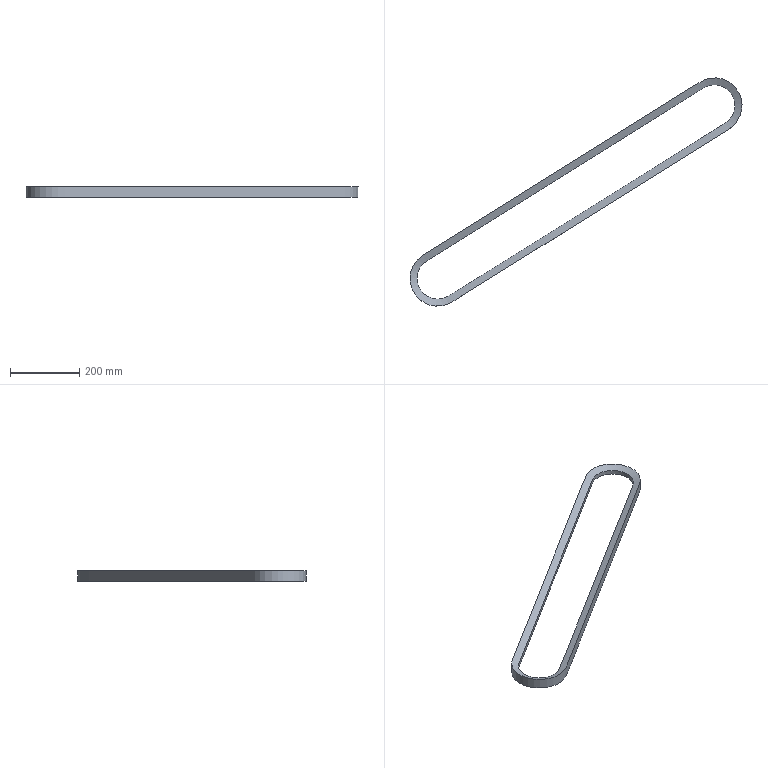Part | NX | 1 solid | 4 faces | box 959.982 x 659.964 x 30 mm | volume 993346 mm3 | spline 4